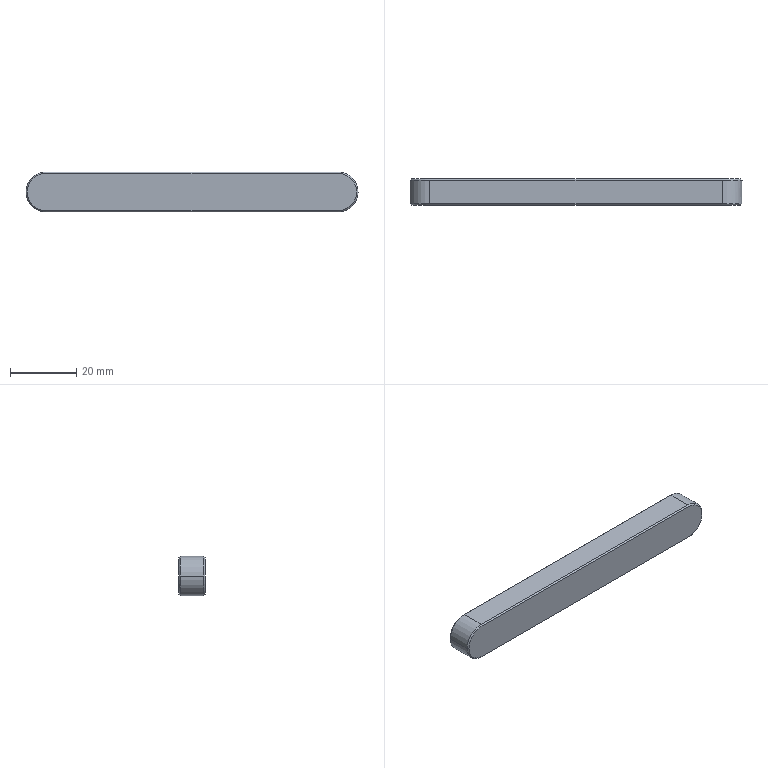Part | STEP file | Input 102 | 1 solid | 17 faces | box 100 x 8 x 12 mm | volume 9319 mm3 | plane 8 | cone 6 | cylinder 3 | commonest cylinder face diameters 12 x3
STEP:
#1=CARTESIAN_POINT('',(0.,0.,0.));
#2=DIRECTION('',(0.,0.,1.));
#3=DIRECTION('',(1.,0.,0.));
#4=AXIS2_PLACEMENT_3D('',#1,#2,#3);
#5=CARTESIAN_POINT('',(3794.6,689.,-0.4063));
#6=VERTEX_POINT('',#5);
#7=CARTESIAN_POINT('',(3789.,689.,-6.006));
#8=VERTEX_POINT('',#7);
#9=CARTESIAN_POINT('',(3789.,689.,-0.4063));
#10=DIRECTION('',(0.,1.,0.));
#11=DIRECTION('',(-1.,0.,0.));
#12=AXIS2_PLACEMENT_3D('',#9,#10,#11);
#13=CIRCLE('',#12,5.6);
#14=CARTESIAN_POINT('',(3789.,689.,-0.4063));
#15=DIRECTION('',(0.,-1.,0.));
#16=DIRECTION('',(1.,0.,0.));
#17=AXIS2_PLACEMENT_3D('',#14,#15,#16);
#18=CONICAL_SURFACE('',#17,5.6,0.7854);
#19=CARTESIAN_POINT('',(9.425,0.));
#20=DIRECTION('',(-1.,0.));
#21=VECTOR('',#20,1.);
#22=LINE('',#19,#21);
#23=(GEOMETRIC_REPRESENTATION_CONTEXT(2)PARAMETRIC_REPRESENTATION_CONTEXT()REPRESENTATION_CONTEXT('',''));
#24=DEFINITIONAL_REPRESENTATION('',(#22),#23);
#25=PCURVE('',#18,#24);
#26=CARTESIAN_POINT('',(3745.,689.,-0.4063));
#27=DIRECTION('',(0.,1.,0.));
#28=DIRECTION('',(-1.,0.,0.));
#29=AXIS2_PLACEMENT_3D('',#26,#27,#28);
#30=PLANE('',#29);
#31=CARTESIAN_POINT('',(-44.,0.));
#32=DIRECTION('',(1.,0.));
#33=AXIS2_PLACEMENT_2D('',#31,#32);
#34=CIRCLE('',#33,5.6);
#35=(GEOMETRIC_REPRESENTATION_CONTEXT(2)PARAMETRIC_REPRESENTATION_CONTEXT()REPRESENTATION_CONTEXT('',''));
#36=DEFINITIONAL_REPRESENTATION('',(#34),#35);
#37=PCURVE('',#30,#36);
#38=SURFACE_CURVE('',#13,(#25,#37),.PCURVE_S1.);
#39=EDGE_CURVE('',#6,#8,#38,.T.);
#40=ORIENTED_EDGE('',*,*,#39,.F.);
#41=CARTESIAN_POINT('',(3795.,688.6,-0.4063));
#42=VERTEX_POINT('',#41);
#43=CARTESIAN_POINT('',(3794.6,689.,-0.4063));
#44=DIRECTION('',(0.7071,-0.7071,0.));
#45=VECTOR('',#44,1.);
#46=LINE('',#43,#45);
#47=CARTESIAN_POINT('',(6.283,0.));
#48=DIRECTION('',(0.,1.));
#49=VECTOR('',#48,1.);
#50=LINE('',#47,#49);
#51=(GEOMETRIC_REPRESENTATION_CONTEXT(2)PARAMETRIC_REPRESENTATION_CONTEXT()REPRESENTATION_CONTEXT('',''));
#52=DEFINITIONAL_REPRESENTATION('',(#50),#51);
#53=PCURVE('',#18,#52);
#54=CARTESIAN_POINT('',(3789.,689.,-0.4063));
#55=DIRECTION('',(0.,-1.,0.));
#56=DIRECTION('',(1.,0.,0.));
#57=AXIS2_PLACEMENT_3D('',#54,#55,#56);
#58=CONICAL_SURFACE('',#57,5.6,0.7854);
#59=CARTESIAN_POINT('',(0.,0.));
#60=DIRECTION('',(0.,1.));
#61=VECTOR('',#60,1.);
#62=LINE('',#59,#61);
#63=(GEOMETRIC_REPRESENTATION_CONTEXT(2)PARAMETRIC_REPRESENTATION_CONTEXT()REPRESENTATION_CONTEXT('',''));
#64=DEFINITIONAL_REPRESENTATION('',(#62),#63);
#65=PCURVE('',#58,#64);
#66=SURFACE_CURVE('',#46,(#53,#65),.PCURVE_S1.);
#67=EDGE_CURVE('',#6,#42,#66,.T.);
#68=ORIENTED_EDGE('',*,*,#67,.T.);
#69=CARTESIAN_POINT('',(3789.,688.6,-6.406));
#70=VERTEX_POINT('',#69);
#71=CARTESIAN_POINT('',(3789.,688.6,-0.4063));
#72=DIRECTION('',(0.,-1.,0.));
#73=DIRECTION('',(-1.,0.,0.));
#74=AXIS2_PLACEMENT_3D('',#71,#72,#73);
#75=CIRCLE('',#74,6.);
#76=CARTESIAN_POINT('',(3.142,0.4));
#77=DIRECTION('',(1.,0.));
#78=VECTOR('',#77,1.);
#79=LINE('',#76,#78);
#80=(GEOMETRIC_REPRESENTATION_CONTEXT(2)PARAMETRIC_REPRESENTATION_CONTEXT()REPRESENTATION_CONTEXT('',''));
#81=DEFINITIONAL_REPRESENTATION('',(#79),#80);
#82=PCURVE('',#18,#81);
#83=CARTESIAN_POINT('',(3789.,681.,-0.4063));
#84=DIRECTION('',(0.,1.,0.));
#85=DIRECTION('',(-1.,0.,0.));
#86=AXIS2_PLACEMENT_3D('',#83,#84,#85);
#87=CYLINDRICAL_SURFACE('',#86,6.);
#88=CARTESIAN_POINT('',(6.283,7.6));
#89=DIRECTION('',(-1.,0.));
#90=VECTOR('',#89,1.);
#91=LINE('',#88,#90);
#92=(GEOMETRIC_REPRESENTATION_CONTEXT(2)PARAMETRIC_REPRESENTATION_CONTEXT()REPRESENTATION_CONTEXT('',''));
#93=DEFINITIONAL_REPRESENTATION('',(#91),#92);
#94=PCURVE('',#87,#93);
#95=SURFACE_CURVE('',#75,(#82,#94),.PCURVE_S1.);
#96=EDGE_CURVE('',#70,#42,#95,.T.);
#97=ORIENTED_EDGE('',*,*,#96,.F.);
#98=CARTESIAN_POINT('',(3789.,688.6,-6.406));
#99=DIRECTION('',(0.,0.7071,0.7071));
#100=VECTOR('',#99,1.);
#101=LINE('',#98,#100);
#102=CARTESIAN_POINT('',(4.712,0.4));
#103=DIRECTION('',(0.,-1.));
#104=VECTOR('',#103,1.);
#105=LINE('',#102,#104);
#106=(GEOMETRIC_REPRESENTATION_CONTEXT(2)PARAMETRIC_REPRESENTATION_CONTEXT()REPRESENTATION_CONTEXT('',''));
#107=DEFINITIONAL_REPRESENTATION('',(#105),#106);
#108=PCURVE('',#18,#107);
#109=CARTESIAN_POINT('',(3745.,688.6,-6.406));
#110=DIRECTION('',(0.,-0.7071,0.7071));
#111=DIRECTION('',(0.,0.7071,0.7071));
#112=AXIS2_PLACEMENT_3D('',#109,#110,#111);
#113=PLANE('',#112);
#114=CARTESIAN_POINT('',(0.,-44.));
#115=DIRECTION('',(1.,0.));
#116=VECTOR('',#115,1.);
#117=LINE('',#114,#116);
#118=(GEOMETRIC_REPRESENTATION_CONTEXT(2)PARAMETRIC_REPRESENTATION_CONTEXT()REPRESENTATION_CONTEXT('',''));
#119=DEFINITIONAL_REPRESENTATION('',(#117),#118);
#120=PCURVE('',#113,#119);
#121=SURFACE_CURVE('',#101,(#108,#120),.PCURVE_S1.);
#122=EDGE_CURVE('',#70,#8,#121,.T.);
#123=ORIENTED_EDGE('',*,*,#122,.T.);
#124=EDGE_LOOP('',(#40,#68,#97,#123));
#125=FACE_BOUND('',#124,.T.);
#126=ADVANCED_FACE('',(#125),#18,.T.);
#127=CARTESIAN_POINT('',(3695.4,681.,-0.4063));
#128=VERTEX_POINT('',#127);
#129=CARTESIAN_POINT('',(3701.,681.,-6.006));
#130=VERTEX_POINT('',#129);
#131=CARTESIAN_POINT('',(3701.,681.,-0.4063));
#132=DIRECTION('',(0.,-1.,0.));
#133=DIRECTION('',(1.,0.,0.));
#134=AXIS2_PLACEMENT_3D('',#131,#132,#133);
#135=CIRCLE('',#134,5.6);
#136=CARTESIAN_POINT('',(3701.,681.,-0.4063));
#137=DIRECTION('',(0.,1.,0.));
#138=DIRECTION('',(-1.,0.,0.));
#139=AXIS2_PLACEMENT_3D('',#136,#137,#138);
#140=CONICAL_SURFACE('',#139,5.6,0.7854);
#141=CARTESIAN_POINT('',(9.425,0.));
#142=DIRECTION('',(-1.,0.));
#143=VECTOR('',#142,1.);
#144=LINE('',#141,#143);
#145=(GEOMETRIC_REPRESENTATION_CONTEXT(2)PARAMETRIC_REPRESENTATION_CONTEXT()REPRESENTATION_CONTEXT('',''));
#146=DEFINITIONAL_REPRESENTATION('',(#144),#145);
#147=PCURVE('',#140,#146);
#148=CARTESIAN_POINT('',(3745.,681.,-0.4063));
#149=DIRECTION('',(0.,-1.,0.));
#150=DIRECTION('',(1.,0.,0.));
#151=AXIS2_PLACEMENT_3D('',#148,#149,#150);
#152=PLANE('',#151);
#153=CARTESIAN_POINT('',(-44.,0.));
#154=DIRECTION('',(1.,0.));
#155=AXIS2_PLACEMENT_2D('',#153,#154);
#156=CIRCLE('',#155,5.6);
#157=(GEOMETRIC_REPRESENTATION_CONTEXT(2)PARAMETRIC_REPRESENTATION_CONTEXT()REPRESENTATION_CONTEXT('',''));
#158=DEFINITIONAL_REPRESENTATION('',(#156),#157);
#159=PCURVE('',#152,#158);
#160=SURFACE_CURVE('',#135,(#147,#159),.PCURVE_S1.);
#161=EDGE_CURVE('',#128,#130,#160,.T.);
#162=ORIENTED_EDGE('',*,*,#161,.F.);
#163=CARTESIAN_POINT('',(3695.,681.4,-0.4063));
#164=VERTEX_POINT('',#163);
#165=CARTESIAN_POINT('',(3695.4,681.,-0.4063));
#166=DIRECTION('',(-0.7071,0.7071,0.));
#167=VECTOR('',#166,1.);
#168=LINE('',#165,#167);
#169=CARTESIAN_POINT('',(6.283,0.));
#170=DIRECTION('',(0.,1.));
#171=VECTOR('',#170,1.);
#172=LINE('',#169,#171);
#173=(GEOMETRIC_REPRESENTATION_CONTEXT(2)PARAMETRIC_REPRESENTATION_CONTEXT()REPRESENTATION_CONTEXT('',''));
#174=DEFINITIONAL_REPRESENTATION('',(#172),#173);
#175=PCURVE('',#140,#174);
#176=CARTESIAN_POINT('',(3701.,681.,-0.4063));
#177=DIRECTION('',(0.,1.,0.));
#178=DIRECTION('',(-1.,0.,0.));
#179=AXIS2_PLACEMENT_3D('',#176,#177,#178);
#180=CONICAL_SURFACE('',#179,5.6,0.7854);
#181=CARTESIAN_POINT('',(0.,0.));
#182=DIRECTION('',(0.,1.));
#183=VECTOR('',#182,1.);
#184=LINE('',#181,#183);
#185=(GEOMETRIC_REPRESENTATION_CONTEXT(2)PARAMETRIC_REPRESENTATION_CONTEXT()REPRESENTATION_CONTEXT('',''));
#186=DEFINITIONAL_REPRESENTATION('',(#184),#185);
#187=PCURVE('',#180,#186);
#188=SURFACE_CURVE('',#168,(#175,#187),.PCURVE_S1.);
#189=EDGE_CURVE('',#128,#164,#188,.T.);
#190=ORIENTED_EDGE('',*,*,#189,.T.);
#191=CARTESIAN_POINT('',(3701.,681.4,-6.406));
#192=VERTEX_POINT('',#191);
#193=CARTESIAN_POINT('',(3701.,681.4,-0.4063));
#194=DIRECTION('',(0.,1.,0.));
#195=DIRECTION('',(1.,0.,0.));
#196=AXIS2_PLACEMENT_3D('',#193,#194,#195);
#197=CIRCLE('',#196,6.);
#198=CARTESIAN_POINT('',(3.142,0.4));
#199=DIRECTION('',(1.,0.));
#200=VECTOR('',#199,1.);
#201=LINE('',#198,#200);
#202=(GEOMETRIC_REPRESENTATION_CONTEXT(2)PARAMETRIC_REPRESENTATION_CONTEXT()REPRESENTATION_CONTEXT('',''));
#203=DEFINITIONAL_REPRESENTATION('',(#201),#202);
#204=PCURVE('',#140,#203);
#205=CARTESIAN_POINT('',(3701.,681.,-0.4063));
#206=DIRECTION('',(0.,1.,0.));
#207=DIRECTION('',(-1.,0.,0.));
#208=AXIS2_PLACEMENT_3D('',#205,#206,#207);
#209=CYLINDRICAL_SURFACE('',#208,6.);
#210=CARTESIAN_POINT('',(3.142,0.4));
#211=DIRECTION('',(1.,0.));
#212=VECTOR('',#211,1.);
#213=LINE('',#210,#212);
#214=(GEOMETRIC_REPRESENTATION_CONTEXT(2)PARAMETRIC_REPRESENTATION_CONTEXT()REPRESENTATION_CONTEXT('',''));
#215=DEFINITIONAL_REPRESENTATION('',(#213),#214);
#216=PCURVE('',#209,#215);
#217=SURFACE_CURVE('',#197,(#204,#216),.PCURVE_S1.);
#218=EDGE_CURVE('',#192,#164,#217,.T.);
#219=ORIENTED_EDGE('',*,*,#218,.F.);
#220=CARTESIAN_POINT('',(3701.,681.4,-6.406));
#221=DIRECTION('',(0.,-0.7071,0.7071));
#222=VECTOR('',#221,1.);
#223=LINE('',#220,#222);
#224=CARTESIAN_POINT('',(4.712,0.4));
#225=DIRECTION('',(0.,-1.));
#226=VECTOR('',#225,1.);
#227=LINE('',#224,#226);
#228=(GEOMETRIC_REPRESENTATION_CONTEXT(2)PARAMETRIC_REPRESENTATION_CONTEXT()REPRESENTATION_CONTEXT('',''));
#229=DEFINITIONAL_REPRESENTATION('',(#227),#228);
#230=PCURVE('',#140,#229);
#231=CARTESIAN_POINT('',(3745.,681.4,-6.406));
#232=DIRECTION('',(0.,0.7071,0.7071));
#233=DIRECTION('',(0.,0.7071,-0.7071));
#234=AXIS2_PLACEMENT_3D('',#231,#232,#233);
#235=PLANE('',#234);
#236=CARTESIAN_POINT('',(0.,44.));
#237=DIRECTION('',(-1.,0.));
#238=VECTOR('',#237,1.);
#239=LINE('',#236,#238);
#240=(GEOMETRIC_REPRESENTATION_CONTEXT(2)PARAMETRIC_REPRESENTATION_CONTEXT()REPRESENTATION_CONTEXT('',''));
#241=DEFINITIONAL_REPRESENTATION('',(#239),#240);
#242=PCURVE('',#235,#241);
#243=SURFACE_CURVE('',#223,(#230,#242),.PCURVE_S1.);
#244=EDGE_CURVE('',#192,#130,#243,.T.);
#245=ORIENTED_EDGE('',*,*,#244,.T.);
#246=EDGE_LOOP('',(#162,#190,#219,#245));
#247=FACE_BOUND('',#246,.T.);
#248=ADVANCED_FACE('',(#247),#140,.T.);
#249=ORIENTED_EDGE('',*,*,#218,.T.);
#250=CARTESIAN_POINT('',(3695.,688.6,-0.4063));
#251=VERTEX_POINT('',#250);
#252=CARTESIAN_POINT('',(3695.,681.,-0.4063));
#253=DIRECTION('',(0.,1.,0.));
#254=VECTOR('',#253,1.);
#255=LINE('',#252,#254);
#256=CARTESIAN_POINT('',(6.283,0.));
#257=DIRECTION('',(0.,1.));
#258=VECTOR('',#257,1.);
#259=LINE('',#256,#258);
#260=(GEOMETRIC_REPRESENTATION_CONTEXT(2)PARAMETRIC_REPRESENTATION_CONTEXT()REPRESENTATION_CONTEXT('',''));
#261=DEFINITIONAL_REPRESENTATION('',(#259),#260);
#262=PCURVE('',#209,#261);
#263=CARTESIAN_POINT('',(3701.,681.,-0.4063));
#264=DIRECTION('',(0.,1.,0.));
#265=DIRECTION('',(-1.,0.,0.));
#266=AXIS2_PLACEMENT_3D('',#263,#264,#265);
#267=CYLINDRICAL_SURFACE('',#266,6.);
#268=CARTESIAN_POINT('',(0.,0.));
#269=DIRECTION('',(0.,1.));
#270=VECTOR('',#269,1.);
#271=LINE('',#268,#270);
#272=(GEOMETRIC_REPRESENTATION_CONTEXT(2)PARAMETRIC_REPRESENTATION_CONTEXT()REPRESENTATION_CONTEXT('',''));
#273=DEFINITIONAL_REPRESENTATION('',(#271),#272);
#274=PCURVE('',#267,#273);
#275=SURFACE_CURVE('',#255,(#262,#274),.PCURVE_S1.);
#276=EDGE_CURVE('',#164,#251,#275,.T.);
#277=ORIENTED_EDGE('',*,*,#276,.T.);
#278=CARTESIAN_POINT('',(3701.,688.6,-6.406));
#279=VERTEX_POINT('',#278);
#280=CARTESIAN_POINT('',(3701.,688.6,-0.4063));
#281=DIRECTION('',(0.,-1.,0.));
#282=DIRECTION('',(-1.,0.,0.));
#283=AXIS2_PLACEMENT_3D('',#280,#281,#282);
#284=CIRCLE('',#283,6.);
#285=CARTESIAN_POINT('',(6.283,7.6));
#286=DIRECTION('',(-1.,0.));
#287=VECTOR('',#286,1.);
#288=LINE('',#285,#287);
#289=(GEOMETRIC_REPRESENTATION_CONTEXT(2)PARAMETRIC_REPRESENTATION_CONTEXT()REPRESENTATION_CONTEXT('',''));
#290=DEFINITIONAL_REPRESENTATION('',(#288),#289);
#291=PCURVE('',#209,#290);
#292=CARTESIAN_POINT('',(3701.,689.,-0.4063));
#293=DIRECTION('',(0.,-1.,0.));
#294=DIRECTION('',(1.,0.,0.));
#295=AXIS2_PLACEMENT_3D('',#292,#293,#294);
#296=CONICAL_SURFACE('',#295,5.6,0.7854);
#297=CARTESIAN_POINT('',(3.142,0.4));
#298=DIRECTION('',(1.,0.));
#299=VECTOR('',#298,1.);
#300=LINE('',#297,#299);
#301=(GEOMETRIC_REPRESENTATION_CONTEXT(2)PARAMETRIC_REPRESENTATION_CONTEXT()REPRESENTATION_CONTEXT('',''));
#302=DEFINITIONAL_REPRESENTATION('',(#300),#301);
#303=PCURVE('',#296,#302);
#304=SURFACE_CURVE('',#284,(#291,#303),.PCURVE_S1.);
#305=EDGE_CURVE('',#251,#279,#304,.T.);
#306=ORIENTED_EDGE('',*,*,#305,.T.);
#307=CARTESIAN_POINT('',(3701.,681.,-6.406));
#308=DIRECTION('',(0.,1.,0.));
#309=VECTOR('',#308,1.);
#310=LINE('',#307,#309);
#311=CARTESIAN_POINT('',(4.712,0.));
#312=DIRECTION('',(0.,1.));
#313=VECTOR('',#312,1.);
#314=LINE('',#311,#313);
#315=(GEOMETRIC_REPRESENTATION_CONTEXT(2)PARAMETRIC_REPRESENTATION_CONTEXT()REPRESENTATION_CONTEXT('',''));
#316=DEFINITIONAL_REPRESENTATION('',(#314),#315);
#317=PCURVE('',#209,#316);
#318=CARTESIAN_POINT('',(3745.,681.,-6.406));
#319=DIRECTION('',(0.,0.,-1.));
#320=DIRECTION('',(0.,-1.,0.));
#321=AXIS2_PLACEMENT_3D('',#318,#319,#320);
#322=PLANE('',#321);
#323=CARTESIAN_POINT('',(0.,44.));
#324=DIRECTION('',(-1.,0.));
#325=VECTOR('',#324,1.);
#326=LINE('',#323,#325);
#327=(GEOMETRIC_REPRESENTATION_CONTEXT(2)PARAMETRIC_REPRESENTATION_CONTEXT()REPRESENTATION_CONTEXT('',''));
#328=DEFINITIONAL_REPRESENTATION('',(#326),#327);
#329=PCURVE('',#322,#328);
#330=SURFACE_CURVE('',#310,(#317,#329),.PCURVE_S1.);
#331=EDGE_CURVE('',#192,#279,#330,.T.);
#332=ORIENTED_EDGE('',*,*,#331,.F.);
#333=EDGE_LOOP('',(#249,#277,#306,#332));
#334=FACE_BOUND('',#333,.T.);
#335=ADVANCED_FACE('',(#334),#209,.T.);
#336=CARTESIAN_POINT('',(3701.,689.,-6.006));
#337=VERTEX_POINT('',#336);
#338=CARTESIAN_POINT('',(3701.,689.,5.194));
#339=VERTEX_POINT('',#338);
#340=CARTESIAN_POINT('',(3701.,689.,-0.4063));
#341=DIRECTION('',(0.,1.,0.));
#342=DIRECTION('',(-1.,0.,0.));
#343=AXIS2_PLACEMENT_3D('',#340,#341,#342);
#344=CIRCLE('',#343,5.6);
#345=CARTESIAN_POINT('',(44.,0.));
#346=DIRECTION('',(1.,0.));
#347=AXIS2_PLACEMENT_2D('',#345,#346);
#348=CIRCLE('',#347,5.6);
#349=(GEOMETRIC_REPRESENTATION_CONTEXT(2)PARAMETRIC_REPRESENTATION_CONTEXT()REPRESENTATION_CONTEXT('',''));
#350=DEFINITIONAL_REPRESENTATION('',(#348),#349);
#351=PCURVE('',#30,#350);
#352=CARTESIAN_POINT('',(9.425,0.));
#353=DIRECTION('',(-1.,0.));
#354=VECTOR('',#353,1.);
#355=LINE('',#352,#354);
#356=(GEOMETRIC_REPRESENTATION_CONTEXT(2)PARAMETRIC_REPRESENTATION_CONTEXT()REPRESENTATION_CONTEXT('',''));
#357=DEFINITIONAL_REPRESENTATION('',(#355),#356);
#358=PCURVE('',#296,#357);
#359=SURFACE_CURVE('',#344,(#351,#358),.PCURVE_S1.);
#360=EDGE_CURVE('',#337,#339,#359,.T.);
#361=ORIENTED_EDGE('',*,*,#360,.T.);
#362=CARTESIAN_POINT('',(3789.,689.,5.194));
#363=VERTEX_POINT('',#362);
#364=CARTESIAN_POINT('',(3745.,689.,5.194));
#365=DIRECTION('',(1.,0.,0.));
#366=VECTOR('',#365,1.);
#367=LINE('',#364,#366);
#368=CARTESIAN_POINT('',(0.,5.6));
#369=DIRECTION('',(-1.,0.));
#370=VECTOR('',#369,1.);
#371=LINE('',#368,#370);
#372=(GEOMETRIC_REPRESENTATION_CONTEXT(2)PARAMETRIC_REPRESENTATION_CONTEXT()REPRESENTATION_CONTEXT('',''));
#373=DEFINITIONAL_REPRESENTATION('',(#371),#372);
#374=PCURVE('',#30,#373);
#375=CARTESIAN_POINT('',(3745.,688.6,5.594));
#376=DIRECTION('',(0.,-0.7071,-0.7071));
#377=DIRECTION('',(0.,-0.7071,0.7071));
#378=AXIS2_PLACEMENT_3D('',#375,#376,#377);
#379=PLANE('',#378);
#380=CARTESIAN_POINT('',(-0.5657,0.));
#381=DIRECTION('',(0.,-1.));
#382=VECTOR('',#381,1.);
#383=LINE('',#380,#382);
#384=(GEOMETRIC_REPRESENTATION_CONTEXT(2)PARAMETRIC_REPRESENTATION_CONTEXT()REPRESENTATION_CONTEXT('',''));
#385=DEFINITIONAL_REPRESENTATION('',(#383),#384);
#386=PCURVE('',#379,#385);
#387=SURFACE_CURVE('',#367,(#374,#386),.PCURVE_S1.);
#388=EDGE_CURVE('',#339,#363,#387,.T.);
#389=ORIENTED_EDGE('',*,*,#388,.T.);
#390=CARTESIAN_POINT('',(3789.,689.,-0.4063));
#391=DIRECTION('',(0.,1.,0.));
#392=DIRECTION('',(-1.,0.,0.));
#393=AXIS2_PLACEMENT_3D('',#390,#391,#392);
#394=CIRCLE('',#393,5.6);
#395=CARTESIAN_POINT('',(-44.,0.));
#396=DIRECTION('',(1.,0.));
#397=AXIS2_PLACEMENT_2D('',#395,#396);
#398=CIRCLE('',#397,5.6);
#399=(GEOMETRIC_REPRESENTATION_CONTEXT(2)PARAMETRIC_REPRESENTATION_CONTEXT()REPRESENTATION_CONTEXT('',''));
#400=DEFINITIONAL_REPRESENTATION('',(#398),#399);
#401=PCURVE('',#30,#400);
#402=CARTESIAN_POINT('',(3.142,0.));
#403=DIRECTION('',(-1.,0.));
#404=VECTOR('',#403,1.);
#405=LINE('',#402,#404);
#406=(GEOMETRIC_REPRESENTATION_CONTEXT(2)PARAMETRIC_REPRESENTATION_CONTEXT()REPRESENTATION_CONTEXT('',''));
#407=DEFINITIONAL_REPRESENTATION('',(#405),#406);
#408=PCURVE('',#58,#407);
#409=SURFACE_CURVE('',#394,(#401,#408),.PCURVE_S1.);
#410=EDGE_CURVE('',#363,#6,#409,.T.);
#411=ORIENTED_EDGE('',*,*,#410,.T.);
#412=ORIENTED_EDGE('',*,*,#39,.T.);
#413=CARTESIAN_POINT('',(3745.,689.,-6.006));
#414=DIRECTION('',(-1.,0.,0.));
#415=VECTOR('',#414,1.);
#416=LINE('',#413,#415);
#417=CARTESIAN_POINT('',(0.,-5.6));
#418=DIRECTION('',(1.,0.));
#419=VECTOR('',#418,1.);
#420=LINE('',#417,#419);
#421=(GEOMETRIC_REPRESENTATION_CONTEXT(2)PARAMETRIC_REPRESENTATION_CONTEXT()REPRESENTATION_CONTEXT('',''));
#422=DEFINITIONAL_REPRESENTATION('',(#420),#421);
#423=PCURVE('',#30,#422);
#424=CARTESIAN_POINT('',(0.5657,0.));
#425=DIRECTION('',(0.,1.));
#426=VECTOR('',#425,1.);
#427=LINE('',#424,#426);
#428=(GEOMETRIC_REPRESENTATION_CONTEXT(2)PARAMETRIC_REPRESENTATION_CONTEXT()REPRESENTATION_CONTEXT('',''));
#429=DEFINITIONAL_REPRESENTATION('',(#427),#428);
#430=PCURVE('',#113,#429);
#431=SURFACE_CURVE('',#416,(#423,#430),.PCURVE_S1.);
#432=EDGE_CURVE('',#8,#337,#431,.T.);
#433=ORIENTED_EDGE('',*,*,#432,.T.);
#434=EDGE_LOOP('',(#361,#389,#411,#412,#433));
#435=FACE_BOUND('',#434,.T.);
#436=ADVANCED_FACE('',(#435),#30,.T.);
#437=CARTESIAN_POINT('',(3789.,681.4,-6.406));
#438=VERTEX_POINT('',#437);
#439=CARTESIAN_POINT('',(3789.,681.,-6.406));
#440=DIRECTION('',(0.,-1.,0.));
#441=VECTOR('',#440,1.);
#442=LINE('',#439,#441);
#443=CARTESIAN_POINT('',(0.,-44.));
#444=DIRECTION('',(1.,0.));
#445=VECTOR('',#444,1.);
#446=LINE('',#443,#445);
#447=(GEOMETRIC_REPRESENTATION_CONTEXT(2)PARAMETRIC_REPRESENTATION_CONTEXT()REPRESENTATION_CONTEXT('',''));
#448=DEFINITIONAL_REPRESENTATION('',(#446),#447);
#449=PCURVE('',#322,#448);
#450=CARTESIAN_POINT('',(4.712,0.));
#451=DIRECTION('',(0.,-1.));
#452=VECTOR('',#451,1.);
#453=LINE('',#450,#452);
#454=(GEOMETRIC_REPRESENTATION_CONTEXT(2)PARAMETRIC_REPRESENTATION_CONTEXT()REPRESENTATION_CONTEXT('',''));
#455=DEFINITIONAL_REPRESENTATION('',(#453),#454);
#456=PCURVE('',#87,#455);
#457=SURFACE_CURVE('',#442,(#449,#456),.PCURVE_S1.);
#458=EDGE_CURVE('',#70,#438,#457,.T.);
#459=ORIENTED_EDGE('',*,*,#458,.T.);
#460=CARTESIAN_POINT('',(3745.,681.4,-6.406));
#461=DIRECTION('',(-1.,0.,0.));
#462=VECTOR('',#461,1.);
#463=LINE('',#460,#462);
#464=CARTESIAN_POINT('',(-0.4,0.));
#465=DIRECTION('',(0.,1.));
#466=VECTOR('',#465,1.);
#467=LINE('',#464,#466);
#468=(GEOMETRIC_REPRESENTATION_CONTEXT(2)PARAMETRIC_REPRESENTATION_CONTEXT()REPRESENTATION_CONTEXT('',''));
#469=DEFINITIONAL_REPRESENTATION('',(#467),#468);
#470=PCURVE('',#322,#469);
#471=CARTESIAN_POINT('',(0.,0.));
#472=DIRECTION('',(0.,1.));
#473=VECTOR('',#472,1.);
#474=LINE('',#471,#473);
#475=(GEOMETRIC_REPRESENTATION_CONTEXT(2)PARAMETRIC_REPRESENTATION_CONTEXT()REPRESENTATION_CONTEXT('',''));
#476=DEFINITIONAL_REPRESENTATION('',(#474),#475);
#477=PCURVE('',#235,#476);
#478=SURFACE_CURVE('',#463,(#470,#477),.PCURVE_S1.);
#479=EDGE_CURVE('',#438,#192,#478,.T.);
#480=ORIENTED_EDGE('',*,*,#479,.T.);
#481=ORIENTED_EDGE('',*,*,#331,.T.);
#482=CARTESIAN_POINT('',(3745.,688.6,-6.406));
#483=DIRECTION('',(1.,0.,0.));
#484=VECTOR('',#483,1.);
#485=LINE('',#482,#484);
#486=CARTESIAN_POINT('',(-7.6,0.));
#487=DIRECTION('',(0.,-1.));
#488=VECTOR('',#487,1.);
#489=LINE('',#486,#488);
#490=(GEOMETRIC_REPRESENTATION_CONTEXT(2)PARAMETRIC_REPRESENTATION_CONTEXT()REPRESENTATION_CONTEXT('',''));
#491=DEFINITIONAL_REPRESENTATION('',(#489),#490);
#492=PCURVE('',#322,#491);
#493=CARTESIAN_POINT('',(0.,0.));
#494=DIRECTION('',(0.,-1.));
#495=VECTOR('',#494,1.);
#496=LINE('',#493,#495);
#497=(GEOMETRIC_REPRESENTATION_CONTEXT(2)PARAMETRIC_REPRESENTATION_CONTEXT()REPRESENTATION_CONTEXT('',''));
#498=DEFINITIONAL_REPRESENTATION('',(#496),#497);
#499=PCURVE('',#113,#498);
#500=SURFACE_CURVE('',#485,(#492,#499),.PCURVE_S1.);
#501=EDGE_CURVE('',#279,#70,#500,.T.);
#502=ORIENTED_EDGE('',*,*,#501,.T.);
#503=EDGE_LOOP('',(#459,#480,#481,#502));
#504=FACE_BOUND('',#503,.T.);
#505=ADVANCED_FACE('',(#504),#322,.T.);
#506=CARTESIAN_POINT('',(3701.,688.6,5.594));
#507=VERTEX_POINT('',#506);
#508=CARTESIAN_POINT('',(3701.,681.4,5.594));
#509=VERTEX_POINT('',#508);
#510=CARTESIAN_POINT('',(3701.,681.,5.594));
#511=DIRECTION('',(0.,-1.,0.));
#512=VECTOR('',#511,1.);
#513=LINE('',#510,#512);
#514=CARTESIAN_POINT('',(3745.,681.,5.594));
#515=DIRECTION('',(0.,0.,1.));
#516=DIRECTION('',(0.,1.,0.));
#517=AXIS2_PLACEMENT_3D('',#514,#515,#516);
#518=PLANE('',#517);
#519=CARTESIAN_POINT('',(0.,44.));
#520=DIRECTION('',(-1.,0.));
#521=VECTOR('',#520,1.);
#522=LINE('',#519,#521);
#523=(GEOMETRIC_REPRESENTATION_CONTEXT(2)PARAMETRIC_REPRESENTATION_CONTEXT()REPRESENTATION_CONTEXT('',''));
#524=DEFINITIONAL_REPRESENTATION('',(#522),#523);
#525=PCURVE('',#518,#524);
#526=CARTESIAN_POINT('',(1.571,0.));
#527=DIRECTION('',(0.,-1.));
#528=VECTOR('',#527,1.);
#529=LINE('',#526,#528);
#530=(GEOMETRIC_REPRESENTATION_CONTEXT(2)PARAMETRIC_REPRESENTATION_CONTEXT()REPRESENTATION_CONTEXT('',''));
#531=DEFINITIONAL_REPRESENTATION('',(#529),#530);
#532=PCURVE('',#267,#531);
#533=SURFACE_CURVE('',#513,(#525,#532),.PCURVE_S1.);
#534=EDGE_CURVE('',#507,#509,#533,.T.);
#535=ORIENTED_EDGE('',*,*,#534,.T.);
#536=CARTESIAN_POINT('',(3789.,681.4,5.594));
#537=VERTEX_POINT('',#536);
#538=CARTESIAN_POINT('',(3745.,681.4,5.594));
#539=DIRECTION('',(1.,0.,0.));
#540=VECTOR('',#539,1.);
#541=LINE('',#538,#540);
#542=CARTESIAN_POINT('',(0.4,0.));
#543=DIRECTION('',(0.,-1.));
#544=VECTOR('',#543,1.);
#545=LINE('',#542,#544);
#546=(GEOMETRIC_REPRESENTATION_CONTEXT(2)PARAMETRIC_REPRESENTATION_CONTEXT()REPRESENTATION_CONTEXT('',''));
#547=DEFINITIONAL_REPRESENTATION('',(#545),#546);
#548=PCURVE('',#518,#547);
#549=CARTESIAN_POINT('',(3745.,681.4,5.594));
#550=DIRECTION('',(0.,0.7071,-0.7071));
#551=DIRECTION('',(0.,-0.7071,-0.7071));
#552=AXIS2_PLACEMENT_3D('',#549,#550,#551);
#553=PLANE('',#552);
#554=CARTESIAN_POINT('',(0.,0.));
#555=DIRECTION('',(0.,-1.));
#556=VECTOR('',#555,1.);
#557=LINE('',#554,#556);
#558=(GEOMETRIC_REPRESENTATION_CONTEXT(2)PARAMETRIC_REPRESENTATION_CONTEXT()REPRESENTATION_CONTEXT('',''));
#559=DEFINITIONAL_REPRESENTATION('',(#557),#558);
#560=PCURVE('',#553,#559);
#561=SURFACE_CURVE('',#541,(#548,#560),.PCURVE_S1.);
#562=EDGE_CURVE('',#509,#537,#561,.T.);
#563=ORIENTED_EDGE('',*,*,#562,.T.);
#564=CARTESIAN_POINT('',(3789.,688.6,5.594));
#565=VERTEX_POINT('',#564);
#566=CARTESIAN_POINT('',(3789.,681.,5.594));
#567=DIRECTION('',(0.,1.,0.));
#568=VECTOR('',#567,1.);
#569=LINE('',#566,#568);
#570=CARTESIAN_POINT('',(0.,-44.));
#571=DIRECTION('',(1.,0.));
#572=VECTOR('',#571,1.);
#573=LINE('',#570,#572);
#574=(GEOMETRIC_REPRESENTATION_CONTEXT(2)PARAMETRIC_REPRESENTATION_CONTEXT()REPRESENTATION_CONTEXT('',''));
#575=DEFINITIONAL_REPRESENTATION('',(#573),#574);
#576=PCURVE('',#518,#575);
#577=CARTESIAN_POINT('',(1.571,0.));
#578=DIRECTION('',(0.,1.));
#579=VECTOR('',#578,1.);
#580=LINE('',#577,#579);
#581=(GEOMETRIC_REPRESENTATION_CONTEXT(2)PARAMETRIC_REPRESENTATION_CONTEXT()REPRESENTATION_CONTEXT('',''));
#582=DEFINITIONAL_REPRESENTATION('',(#580),#581);
#583=PCURVE('',#87,#582);
#584=SURFACE_CURVE('',#569,(#576,#583),.PCURVE_S1.);
#585=EDGE_CURVE('',#537,#565,#584,.T.);
#586=ORIENTED_EDGE('',*,*,#585,.T.);
#587=CARTESIAN_POINT('',(3745.,688.6,5.594));
#588=DIRECTION('',(-1.,0.,0.));
#589=VECTOR('',#588,1.);
#590=LINE('',#587,#589);
#591=CARTESIAN_POINT('',(7.6,0.));
#592=DIRECTION('',(0.,1.));
#593=VECTOR('',#592,1.);
#594=LINE('',#591,#593);
#595=(GEOMETRIC_REPRESENTATION_CONTEXT(2)PARAMETRIC_REPRESENTATION_CONTEXT()REPRESENTATION_CONTEXT('',''));
#596=DEFINITIONAL_REPRESENTATION('',(#594),#595);
#597=PCURVE('',#518,#596);
#598=CARTESIAN_POINT('',(0.,0.));
#599=DIRECTION('',(0.,1.));
#600=VECTOR('',#599,1.);
#601=LINE('',#598,#600);
#602=(GEOMETRIC_REPRESENTATION_CONTEXT(2)PARAMETRIC_REPRESENTATION_CONTEXT()REPRESENTATION_CONTEXT('',''));
#603=DEFINITIONAL_REPRESENTATION('',(#601),#602);
#604=PCURVE('',#379,#603);
#605=SURFACE_CURVE('',#590,(#597,#604),.PCURVE_S1.);
#606=EDGE_CURVE('',#565,#507,#605,.T.);
#607=ORIENTED_EDGE('',*,*,#606,.T.);
#608=EDGE_LOOP('',(#535,#563,#586,#607));
#609=FACE_BOUND('',#608,.T.);
#610=ADVANCED_FACE('',(#609),#518,.T.);
#611=CARTESIAN_POINT('',(3789.,681.,5.194));
#612=VERTEX_POINT('',#611);
#613=CARTESIAN_POINT('',(3701.,681.,5.194));
#614=VERTEX_POINT('',#613);
#615=CARTESIAN_POINT('',(3745.,681.,5.194));
#616=DIRECTION('',(-1.,0.,0.));
#617=VECTOR('',#616,1.);
#618=LINE('',#615,#617);
#619=CARTESIAN_POINT('',(0.,5.6));
#620=DIRECTION('',(-1.,0.));
#621=VECTOR('',#620,1.);
#622=LINE('',#619,#621);
#623=(GEOMETRIC_REPRESENTATION_CONTEXT(2)PARAMETRIC_REPRESENTATION_CONTEXT()REPRESENTATION_CONTEXT('',''));
#624=DEFINITIONAL_REPRESENTATION('',(#622),#623);
#625=PCURVE('',#152,#624);
#626=CARTESIAN_POINT('',(0.5657,0.));
#627=DIRECTION('',(0.,1.));
#628=VECTOR('',#627,1.);
#629=LINE('',#626,#628);
#630=(GEOMETRIC_REPRESENTATION_CONTEXT(2)PARAMETRIC_REPRESENTATION_CONTEXT()REPRESENTATION_CONTEXT('',''));
#631=DEFINITIONAL_REPRESENTATION('',(#629),#630);
#632=PCURVE('',#553,#631);
#633=SURFACE_CURVE('',#618,(#625,#632),.PCURVE_S1.);
#634=EDGE_CURVE('',#612,#614,#633,.T.);
#635=ORIENTED_EDGE('',*,*,#634,.T.);
#636=CARTESIAN_POINT('',(3701.,681.,-0.4063));
#637=DIRECTION('',(0.,-1.,0.));
#638=DIRECTION('',(1.,0.,0.));
#639=AXIS2_PLACEMENT_3D('',#636,#637,#638);
#640=CIRCLE('',#639,5.6);
#641=CARTESIAN_POINT('',(-44.,0.));
#642=DIRECTION('',(1.,0.));
#643=AXIS2_PLACEMENT_2D('',#641,#642);
#644=CIRCLE('',#643,5.6);
#645=(GEOMETRIC_REPRESENTATION_CONTEXT(2)PARAMETRIC_REPRESENTATION_CONTEXT()REPRESENTATION_CONTEXT('',''));
#646=DEFINITIONAL_REPRESENTATION('',(#644),#645);
#647=PCURVE('',#152,#646);
#648=CARTESIAN_POINT('',(3.142,0.));
#649=DIRECTION('',(-1.,0.));
#650=VECTOR('',#649,1.);
#651=LINE('',#648,#650);
#652=(GEOMETRIC_REPRESENTATION_CONTEXT(2)PARAMETRIC_REPRESENTATION_CONTEXT()REPRESENTATION_CONTEXT('',''));
#653=DEFINITIONAL_REPRESENTATION('',(#651),#652);
#654=PCURVE('',#180,#653);
#655=SURFACE_CURVE('',#640,(#647,#654),.PCURVE_S1.);
#656=EDGE_CURVE('',#614,#128,#655,.T.);
#657=ORIENTED_EDGE('',*,*,#656,.T.);
#658=ORIENTED_EDGE('',*,*,#161,.T.);
#659=CARTESIAN_POINT('',(3789.,681.,-6.006));
#660=VERTEX_POINT('',#659);
#661=CARTESIAN_POINT('',(3745.,681.,-6.006));
#662=DIRECTION('',(1.,0.,0.));
#663=VECTOR('',#662,1.);
#664=LINE('',#661,#663);
#665=CARTESIAN_POINT('',(0.,-5.6));
#666=DIRECTION('',(1.,0.));
#667=VECTOR('',#666,1.);
#668=LINE('',#665,#667);
#669=(GEOMETRIC_REPRESENTATION_CONTEXT(2)PARAMETRIC_REPRESENTATION_CONTEXT()REPRESENTATION_CONTEXT('',''));
#670=DEFINITIONAL_REPRESENTATION('',(#668),#669);
#671=PCURVE('',#152,#670);
#672=CARTESIAN_POINT('',(-0.5657,0.));
#673=DIRECTION('',(0.,-1.));
#674=VECTOR('',#673,1.);
#675=LINE('',#672,#674);
#676=(GEOMETRIC_REPRESENTATION_CONTEXT(2)PARAMETRIC_REPRESENTATION_CONTEXT()REPRESENTATION_CONTEXT('',''));
#677=DEFINITIONAL_REPRESENTATION('',(#675),#676);
#678=PCURVE('',#235,#677);
#679=SURFACE_CURVE('',#664,(#671,#678),.PCURVE_S1.);
#680=EDGE_CURVE('',#130,#660,#679,.T.);
#681=ORIENTED_EDGE('',*,*,#680,.T.);
#682=CARTESIAN_POINT('',(3789.,681.,-0.4063));
#683=DIRECTION('',(0.,-1.,0.));
#684=DIRECTION('',(1.,0.,0.));
#685=AXIS2_PLACEMENT_3D('',#682,#683,#684);
#686=CIRCLE('',#685,5.6);
#687=CARTESIAN_POINT('',(44.,0.));
#688=DIRECTION('',(1.,0.));
#689=AXIS2_PLACEMENT_2D('',#687,#688);
#690=CIRCLE('',#689,5.6);
#691=(GEOMETRIC_REPRESENTATION_CONTEXT(2)PARAMETRIC_REPRESENTATION_CONTEXT()REPRESENTATION_CONTEXT('',''));
#692=DEFINITIONAL_REPRESENTATION('',(#690),#691);
#693=PCURVE('',#152,#692);
#694=CARTESIAN_POINT('',(3789.,681.,-0.4063));
#695=DIRECTION('',(0.,1.,0.));
#696=DIRECTION('',(-1.,0.,0.));
#697=AXIS2_PLACEMENT_3D('',#694,#695,#696);
#698=CONICAL_SURFACE('',#697,5.6,0.7854);
#699=CARTESIAN_POINT('',(9.425,0.));
#700=DIRECTION('',(-1.,0.));
#701=VECTOR('',#700,1.);
#702=LINE('',#699,#701);
#703=(GEOMETRIC_REPRESENTATION_CONTEXT(2)PARAMETRIC_REPRESENTATION_CONTEXT()REPRESENTATION_CONTEXT('',''));
#704=DEFINITIONAL_REPRESENTATION('',(#702),#703);
#705=PCURVE('',#698,#704);
#706=SURFACE_CURVE('',#686,(#693,#705),.PCURVE_S1.);
#707=EDGE_CURVE('',#660,#612,#706,.T.);
#708=ORIENTED_EDGE('',*,*,#707,.T.);
#709=EDGE_LOOP('',(#635,#657,#658,#681,#708));
#710=FACE_BOUND('',#709,.T.);
#711=ADVANCED_FACE('',(#710),#152,.T.);
#712=ORIENTED_EDGE('',*,*,#585,.F.);
#713=CARTESIAN_POINT('',(3789.,681.4,-0.4063));
#714=DIRECTION('',(0.,1.,0.));
#715=DIRECTION('',(1.,0.,0.));
#716=AXIS2_PLACEMENT_3D('',#713,#714,#715);
#717=CIRCLE('',#716,6.);
#718=CARTESIAN_POINT('',(-3.142,0.4));
#719=DIRECTION('',(1.,0.));
#720=VECTOR('',#719,1.);
#721=LINE('',#718,#720);
#722=(GEOMETRIC_REPRESENTATION_CONTEXT(2)PARAMETRIC_REPRESENTATION_CONTEXT()REPRESENTATION_CONTEXT('',''));
#723=DEFINITIONAL_REPRESENTATION('',(#721),#722);
#724=PCURVE('',#87,#723);
#725=CARTESIAN_POINT('',(-3.142,0.4));
#726=DIRECTION('',(1.,0.));
#727=VECTOR('',#726,1.);
#728=LINE('',#725,#727);
#729=(GEOMETRIC_REPRESENTATION_CONTEXT(2)PARAMETRIC_REPRESENTATION_CONTEXT()REPRESENTATION_CONTEXT('',''));
#730=DEFINITIONAL_REPRESENTATION('',(#728),#729);
#731=PCURVE('',#698,#730);
#732=SURFACE_CURVE('',#717,(#724,#731),.PCURVE_S1.);
#733=EDGE_CURVE('',#537,#438,#732,.T.);
#734=ORIENTED_EDGE('',*,*,#733,.T.);
#735=ORIENTED_EDGE('',*,*,#458,.F.);
#736=ORIENTED_EDGE('',*,*,#96,.T.);
#737=CARTESIAN_POINT('',(3789.,688.6,-0.4063));
#738=DIRECTION('',(0.,-1.,0.));
#739=DIRECTION('',(-1.,0.,0.));
#740=AXIS2_PLACEMENT_3D('',#737,#738,#739);
#741=CIRCLE('',#740,6.);
#742=CARTESIAN_POINT('',(6.283,7.6));
#743=DIRECTION('',(-1.,0.));
#744=VECTOR('',#743,1.);
#745=LINE('',#742,#744);
#746=(GEOMETRIC_REPRESENTATION_CONTEXT(2)PARAMETRIC_REPRESENTATION_CONTEXT()REPRESENTATION_CONTEXT('',''));
#747=DEFINITIONAL_REPRESENTATION('',(#745),#746);
#748=PCURVE('',#87,#747);
#749=CARTESIAN_POINT('',(-3.142,0.4));
#750=DIRECTION('',(1.,0.));
#751=VECTOR('',#750,1.);
#752=LINE('',#749,#751);
#753=(GEOMETRIC_REPRESENTATION_CONTEXT(2)PARAMETRIC_REPRESENTATION_CONTEXT()REPRESENTATION_CONTEXT('',''));
#754=DEFINITIONAL_REPRESENTATION('',(#752),#753);
#755=PCURVE('',#58,#754);
#756=SURFACE_CURVE('',#741,(#748,#755),.PCURVE_S1.);
#757=EDGE_CURVE('',#42,#565,#756,.T.);
#758=ORIENTED_EDGE('',*,*,#757,.T.);
#759=EDGE_LOOP('',(#712,#734,#735,#736,#758));
#760=FACE_BOUND('',#759,.T.);
#761=ADVANCED_FACE('',(#760),#87,.T.);
#762=ORIENTED_EDGE('',*,*,#276,.F.);
#763=CARTESIAN_POINT('',(3701.,681.4,-0.4063));
#764=DIRECTION('',(0.,1.,0.));
#765=DIRECTION('',(1.,0.,0.));
#766=AXIS2_PLACEMENT_3D('',#763,#764,#765);
#767=CIRCLE('',#766,6.);
#768=CARTESIAN_POINT('',(-3.142,0.4));
#769=DIRECTION('',(1.,0.));
#770=VECTOR('',#769,1.);
#771=LINE('',#768,#770);
#772=(GEOMETRIC_REPRESENTATION_CONTEXT(2)PARAMETRIC_REPRESENTATION_CONTEXT()REPRESENTATION_CONTEXT('',''));
#773=DEFINITIONAL_REPRESENTATION('',(#771),#772);
#774=PCURVE('',#267,#773);
#775=CARTESIAN_POINT('',(-3.142,0.4));
#776=DIRECTION('',(1.,0.));
#777=VECTOR('',#776,1.);
#778=LINE('',#775,#777);
#779=(GEOMETRIC_REPRESENTATION_CONTEXT(2)PARAMETRIC_REPRESENTATION_CONTEXT()REPRESENTATION_CONTEXT('',''));
#780=DEFINITIONAL_REPRESENTATION('',(#778),#779);
#781=PCURVE('',#180,#780);
#782=SURFACE_CURVE('',#767,(#774,#781),.PCURVE_S1.);
#783=EDGE_CURVE('',#164,#509,#782,.T.);
#784=ORIENTED_EDGE('',*,*,#783,.T.);
#785=ORIENTED_EDGE('',*,*,#534,.F.);
#786=CARTESIAN_POINT('',(3701.,688.6,-0.4063));
#787=DIRECTION('',(0.,-1.,0.));
#788=DIRECTION('',(-1.,0.,0.));
#789=AXIS2_PLACEMENT_3D('',#786,#787,#788);
#790=CIRCLE('',#789,6.);
#791=CARTESIAN_POINT('',(6.283,7.6));
#792=DIRECTION('',(-1.,0.));
#793=VECTOR('',#792,1.);
#794=LINE('',#791,#793);
#795=(GEOMETRIC_REPRESENTATION_CONTEXT(2)PARAMETRIC_REPRESENTATION_CONTEXT()REPRESENTATION_CONTEXT('',''));
#796=DEFINITIONAL_REPRESENTATION('',(#794),#795);
#797=PCURVE('',#267,#796);
#798=CARTESIAN_POINT('',(-3.142,0.4));
#799=DIRECTION('',(1.,0.));
#800=VECTOR('',#799,1.);
#801=LINE('',#798,#800);
#802=(GEOMETRIC_REPRESENTATION_CONTEXT(2)PARAMETRIC_REPRESENTATION_CONTEXT()REPRESENTATION_CONTEXT('',''));
#803=DEFINITIONAL_REPRESENTATION('',(#801),#802);
#804=PCURVE('',#296,#803);
#805=SURFACE_CURVE('',#790,(#797,#804),.PCURVE_S1.);
#806=EDGE_CURVE('',#507,#251,#805,.T.);
#807=ORIENTED_EDGE('',*,*,#806,.T.);
#808=EDGE_LOOP('',(#762,#784,#785,#807));
#809=FACE_BOUND('',#808,.T.);
#810=ADVANCED_FACE('',(#809),#267,.T.);
#811=CARTESIAN_POINT('',(3789.,681.4,-6.406));
#812=DIRECTION('',(0.,-0.7071,0.7071));
#813=VECTOR('',#812,1.);
#814=LINE('',#811,#813);
#815=CARTESIAN_POINT('',(4.712,0.4));
#816=DIRECTION('',(0.,-1.));
#817=VECTOR('',#816,1.);
#818=LINE('',#815,#817);
#819=(GEOMETRIC_REPRESENTATION_CONTEXT(2)PARAMETRIC_REPRESENTATION_CONTEXT()REPRESENTATION_CONTEXT('',''));
#820=DEFINITIONAL_REPRESENTATION('',(#818),#819);
#821=PCURVE('',#698,#820);
#822=CARTESIAN_POINT('',(0.,-44.));
#823=DIRECTION('',(-1.,0.));
#824=VECTOR('',#823,1.);
#825=LINE('',#822,#824);
#826=(GEOMETRIC_REPRESENTATION_CONTEXT(2)PARAMETRIC_REPRESENTATION_CONTEXT()REPRESENTATION_CONTEXT('',''));
#827=DEFINITIONAL_REPRESENTATION('',(#825),#826);
#828=PCURVE('',#235,#827);
#829=SURFACE_CURVE('',#814,(#821,#828),.PCURVE_S1.);
#830=EDGE_CURVE('',#438,#660,#829,.T.);
#831=ORIENTED_EDGE('',*,*,#830,.F.);
#832=ORIENTED_EDGE('',*,*,#733,.F.);
#833=CARTESIAN_POINT('',(3789.,681.,5.194));
#834=DIRECTION('',(0.,0.7071,0.7071));
#835=VECTOR('',#834,1.);
#836=LINE('',#833,#835);
#837=CARTESIAN_POINT('',(1.571,0.));
#838=DIRECTION('',(0.,1.));
#839=VECTOR('',#838,1.);
#840=LINE('',#837,#839);
#841=(GEOMETRIC_REPRESENTATION_CONTEXT(2)PARAMETRIC_REPRESENTATION_CONTEXT()REPRESENTATION_CONTEXT('',''));
#842=DEFINITIONAL_REPRESENTATION('',(#840),#841);
#843=PCURVE('',#698,#842);
#844=CARTESIAN_POINT('',(0.5657,-44.));
#845=DIRECTION('',(-1.,0.));
#846=VECTOR('',#845,1.);
#847=LINE('',#844,#846);
#848=(GEOMETRIC_REPRESENTATION_CONTEXT(2)PARAMETRIC_REPRESENTATION_CONTEXT()REPRESENTATION_CONTEXT('',''));
#849=DEFINITIONAL_REPRESENTATION('',(#847),#848);
#850=PCURVE('',#553,#849);
#851=SURFACE_CURVE('',#836,(#843,#850),.PCURVE_S1.);
#852=EDGE_CURVE('',#612,#537,#851,.T.);
#853=ORIENTED_EDGE('',*,*,#852,.F.);
#854=ORIENTED_EDGE('',*,*,#707,.F.);
#855=EDGE_LOOP('',(#831,#832,#853,#854));
#856=FACE_BOUND('',#855,.T.);
#857=ADVANCED_FACE('',(#856),#698,.T.);
#858=ORIENTED_EDGE('',*,*,#852,.T.);
#859=ORIENTED_EDGE('',*,*,#562,.F.);
#860=CARTESIAN_POINT('',(3701.,681.,5.194));
#861=DIRECTION('',(0.,0.7071,0.7071));
#862=VECTOR('',#861,1.);
#863=LINE('',#860,#862);
#864=CARTESIAN_POINT('',(0.5657,44.));
#865=DIRECTION('',(-1.,0.));
#866=VECTOR('',#865,1.);
#867=LINE('',#864,#866);
#868=(GEOMETRIC_REPRESENTATION_CONTEXT(2)PARAMETRIC_REPRESENTATION_CONTEXT()REPRESENTATION_CONTEXT('',''));
#869=DEFINITIONAL_REPRESENTATION('',(#867),#868);
#870=PCURVE('',#553,#869);
#871=CARTESIAN_POINT('',(1.571,0.));
#872=DIRECTION('',(0.,1.));
#873=VECTOR('',#872,1.);
#874=LINE('',#871,#873);
#875=(GEOMETRIC_REPRESENTATION_CONTEXT(2)PARAMETRIC_REPRESENTATION_CONTEXT()REPRESENTATION_CONTEXT('',''));
#876=DEFINITIONAL_REPRESENTATION('',(#874),#875);
#877=PCURVE('',#180,#876);
#878=SURFACE_CURVE('',#863,(#870,#877),.PCURVE_S1.);
#879=EDGE_CURVE('',#614,#509,#878,.T.);
#880=ORIENTED_EDGE('',*,*,#879,.F.);
#881=ORIENTED_EDGE('',*,*,#634,.F.);
#882=EDGE_LOOP('',(#858,#859,#880,#881));
#883=FACE_BOUND('',#882,.T.);
#884=ADVANCED_FACE('',(#883),#553,.F.);
#885=ORIENTED_EDGE('',*,*,#830,.T.);
#886=ORIENTED_EDGE('',*,*,#680,.F.);
#887=ORIENTED_EDGE('',*,*,#244,.F.);
#888=ORIENTED_EDGE('',*,*,#479,.F.);
#889=EDGE_LOOP('',(#885,#886,#887,#888));
#890=FACE_BOUND('',#889,.T.);
#891=ADVANCED_FACE('',(#890),#235,.F.);
#892=ORIENTED_EDGE('',*,*,#189,.F.);
#893=ORIENTED_EDGE('',*,*,#656,.F.);
#894=ORIENTED_EDGE('',*,*,#879,.T.);
#895=ORIENTED_EDGE('',*,*,#783,.F.);
#896=EDGE_LOOP('',(#892,#893,#894,#895));
#897=FACE_BOUND('',#896,.T.);
#898=ADVANCED_FACE('',(#897),#180,.T.);
#899=CARTESIAN_POINT('',(3701.,689.,-6.006));
#900=DIRECTION('',(0.,-0.7071,-0.7071));
#901=VECTOR('',#900,1.);
#902=LINE('',#899,#901);
#903=CARTESIAN_POINT('',(0.5657,44.));
#904=DIRECTION('',(-1.,0.));
#905=VECTOR('',#904,1.);
#906=LINE('',#903,#905);
#907=(GEOMETRIC_REPRESENTATION_CONTEXT(2)PARAMETRIC_REPRESENTATION_CONTEXT()REPRESENTATION_CONTEXT('',''));
#908=DEFINITIONAL_REPRESENTATION('',(#906),#907);
#909=PCURVE('',#113,#908);
#910=CARTESIAN_POINT('',(4.712,0.));
#911=DIRECTION('',(0.,1.));
#912=VECTOR('',#911,1.);
#913=LINE('',#910,#912);
#914=(GEOMETRIC_REPRESENTATION_CONTEXT(2)PARAMETRIC_REPRESENTATION_CONTEXT()REPRESENTATION_CONTEXT('',''));
#915=DEFINITIONAL_REPRESENTATION('',(#913),#914);
#916=PCURVE('',#296,#915);
#917=SURFACE_CURVE('',#902,(#909,#916),.PCURVE_S1.);
#918=EDGE_CURVE('',#337,#279,#917,.T.);
#919=ORIENTED_EDGE('',*,*,#918,.F.);
#920=ORIENTED_EDGE('',*,*,#432,.F.);
#921=ORIENTED_EDGE('',*,*,#122,.F.);
#922=ORIENTED_EDGE('',*,*,#501,.F.);
#923=EDGE_LOOP('',(#919,#920,#921,#922));
#924=FACE_BOUND('',#923,.T.);
#925=ADVANCED_FACE('',(#924),#113,.F.);
#926=ORIENTED_EDGE('',*,*,#67,.F.);
#927=ORIENTED_EDGE('',*,*,#410,.F.);
#928=CARTESIAN_POINT('',(3789.,688.6,5.594));
#929=DIRECTION('',(0.,0.7071,-0.7071));
#930=VECTOR('',#929,1.);
#931=LINE('',#928,#930);
#932=CARTESIAN_POINT('',(1.571,0.4));
#933=DIRECTION('',(0.,-1.));
#934=VECTOR('',#933,1.);
#935=LINE('',#932,#934);
#936=(GEOMETRIC_REPRESENTATION_CONTEXT(2)PARAMETRIC_REPRESENTATION_CONTEXT()REPRESENTATION_CONTEXT('',''));
#937=DEFINITIONAL_REPRESENTATION('',(#935),#936);
#938=PCURVE('',#58,#937);
#939=CARTESIAN_POINT('',(0.,-44.));
#940=DIRECTION('',(-1.,0.));
#941=VECTOR('',#940,1.);
#942=LINE('',#939,#941);
#943=(GEOMETRIC_REPRESENTATION_CONTEXT(2)PARAMETRIC_REPRESENTATION_CONTEXT()REPRESENTATION_CONTEXT('',''));
#944=DEFINITIONAL_REPRESENTATION('',(#942),#943);
#945=PCURVE('',#379,#944);
#946=SURFACE_CURVE('',#931,(#938,#945),.PCURVE_S1.);
#947=EDGE_CURVE('',#565,#363,#946,.T.);
#948=ORIENTED_EDGE('',*,*,#947,.F.);
#949=ORIENTED_EDGE('',*,*,#757,.F.);
#950=EDGE_LOOP('',(#926,#927,#948,#949));
#951=FACE_BOUND('',#950,.T.);
#952=ADVANCED_FACE('',(#951),#58,.T.);
#953=ORIENTED_EDGE('',*,*,#918,.T.);
#954=ORIENTED_EDGE('',*,*,#305,.F.);
#955=ORIENTED_EDGE('',*,*,#806,.F.);
#956=CARTESIAN_POINT('',(3701.,689.,5.194));
#957=DIRECTION('',(0.,-0.7071,0.7071));
#958=VECTOR('',#957,1.);
#959=LINE('',#956,#958);
#960=CARTESIAN_POINT('',(1.571,0.));
#961=DIRECTION('',(0.,1.));
#962=VECTOR('',#961,1.);
#963=LINE('',#960,#962);
#964=(GEOMETRIC_REPRESENTATION_CONTEXT(2)PARAMETRIC_REPRESENTATION_CONTEXT()REPRESENTATION_CONTEXT('',''));
#965=DEFINITIONAL_REPRESENTATION('',(#963),#964);
#966=PCURVE('',#296,#965);
#967=CARTESIAN_POINT('',(-0.5657,44.));
#968=DIRECTION('',(1.,0.));
#969=VECTOR('',#968,1.);
#970=LINE('',#967,#969);
#971=(GEOMETRIC_REPRESENTATION_CONTEXT(2)PARAMETRIC_REPRESENTATION_CONTEXT()REPRESENTATION_CONTEXT('',''));
#972=DEFINITIONAL_REPRESENTATION('',(#970),#971);
#973=PCURVE('',#379,#972);
#974=SURFACE_CURVE('',#959,(#966,#973),.PCURVE_S1.);
#975=EDGE_CURVE('',#339,#507,#974,.T.);
#976=ORIENTED_EDGE('',*,*,#975,.F.);
#977=ORIENTED_EDGE('',*,*,#360,.F.);
#978=EDGE_LOOP('',(#953,#954,#955,#976,#977));
#979=FACE_BOUND('',#978,.T.);
#980=ADVANCED_FACE('',(#979),#296,.T.);
#981=ORIENTED_EDGE('',*,*,#947,.T.);
#982=ORIENTED_EDGE('',*,*,#388,.F.);
#983=ORIENTED_EDGE('',*,*,#975,.T.);
#984=ORIENTED_EDGE('',*,*,#606,.F.);
#985=EDGE_LOOP('',(#981,#982,#983,#984));
#986=FACE_BOUND('',#985,.T.);
#987=ADVANCED_FACE('',(#986),#379,.F.);
#988=CLOSED_SHELL('',(#126,#248,#335,#436,#505,#610,#711,#761,#810,#857,#884,#891,#898,#925,#952,#980,#987));
#989=MANIFOLD_SOLID_BREP('',#988);
#990=(LENGTH_UNIT()NAMED_UNIT(*)SI_UNIT(.MILLI.,.METRE.));
#991=UNCERTAINTY_MEASURE_WITH_UNIT(LENGTH_MEASURE(0.0000001),#990,'','');
#992=(NAMED_UNIT(*)PLANE_ANGLE_UNIT()SI_UNIT($,.RADIAN.));
#993=(NAMED_UNIT(*)SI_UNIT($,.STERADIAN.)SOLID_ANGLE_UNIT());
#994=(GEOMETRIC_REPRESENTATION_CONTEXT(3)GLOBAL_UNCERTAINTY_ASSIGNED_CONTEXT((#991))GLOBAL_UNIT_ASSIGNED_CONTEXT((#990,#992,#993))REPRESENTATION_CONTEXT('',''));
#995=ADVANCED_BREP_SHAPE_REPRESENTATION('',(#4,#989),#994);